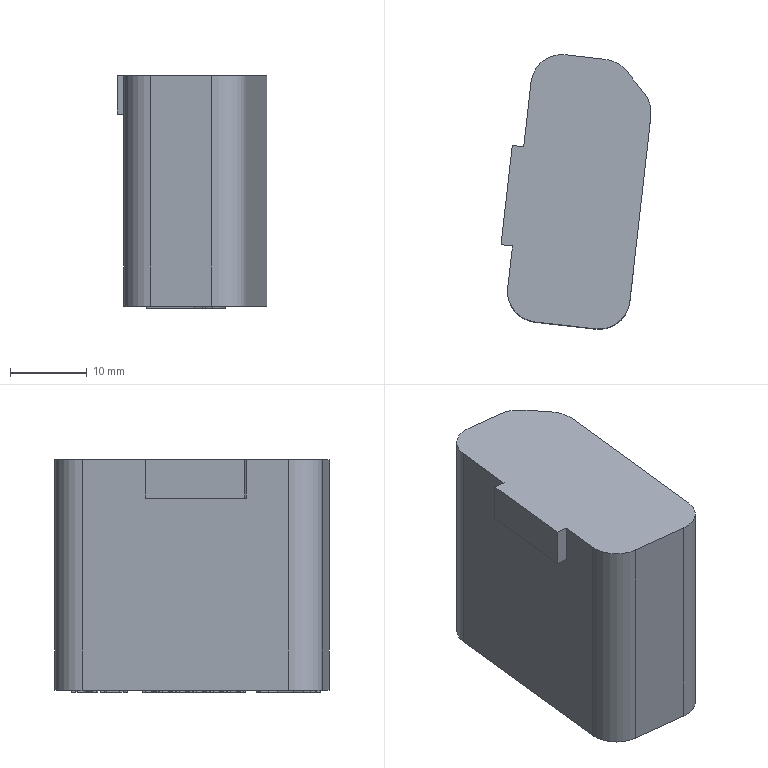Part | NX | features 13 2 | 1 solid | 138 faces | box 19.534 x 35.729 x 30.299 mm | volume 16207 mm3 | plane 103 | spline 28 | cylinder 7 | commonest cylinder face diameters 8 x5 21.767 x1 23.767 x1